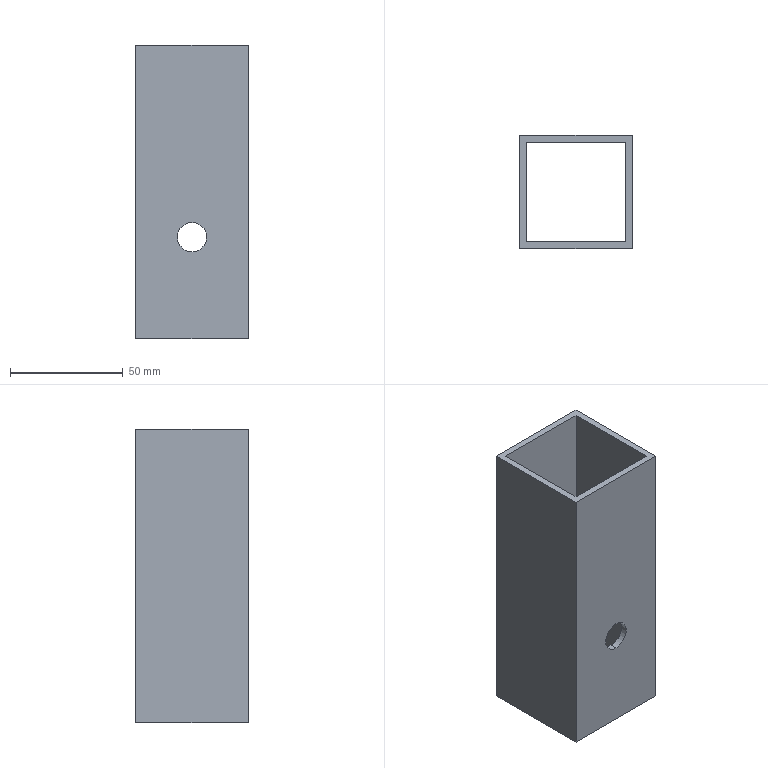Part | SolidWorks | features Cut 1, Extrusion 1 | 1 solid | 14 faces | box 50 x 50 x 130 mm | volume 72524 mm3 | plane 10 | cylinder 4 | commonest cylinder face diameters 13 x4
STEP:
#1=CARTESIAN_POINT('',(25.,0.,38.5));
#2=VERTEX_POINT('',#1);
#3=CARTESIAN_POINT('',(25.,0.,51.5));
#4=VERTEX_POINT('',#3);
#5=CARTESIAN_POINT('',(25.,0.,45.));
#6=DIRECTION('',(0.,1.,0.));
#7=DIRECTION('',(0.,0.,1.));
#8=AXIS2_PLACEMENT_3D('',#5,#6,#7);
#9=CIRCLE('',#8,6.5);
#10=EDGE_CURVE('',#2,#4,#9,.T.);
#11=ORIENTED_EDGE('',*,*,#10,.F.);
#12=CARTESIAN_POINT('',(25.,3.,38.5));
#13=VERTEX_POINT('',#12);
#14=CARTESIAN_POINT('',(25.,-80.,38.5));
#15=DIRECTION('',(0.,1.,0.));
#16=VECTOR('',#15,1000.);
#17=LINE('',#14,#16);
#18=EDGE_CURVE('',#2,#13,#17,.T.);
#19=ORIENTED_EDGE('',*,*,#18,.T.);
#20=CARTESIAN_POINT('',(25.,3.,51.5));
#21=VERTEX_POINT('',#20);
#22=CARTESIAN_POINT('',(25.,3.,45.));
#23=DIRECTION('',(0.,1.,0.));
#24=DIRECTION('',(0.,0.,1.));
#25=AXIS2_PLACEMENT_3D('',#22,#23,#24);
#26=CIRCLE('',#25,6.5);
#27=EDGE_CURVE('',#13,#21,#26,.T.);
#28=ORIENTED_EDGE('',*,*,#27,.T.);
#29=CARTESIAN_POINT('',(25.,-80.,51.5));
#30=DIRECTION('',(0.,1.,0.));
#31=VECTOR('',#30,1000.);
#32=LINE('',#29,#31);
#33=EDGE_CURVE('',#4,#21,#32,.T.);
#34=ORIENTED_EDGE('',*,*,#33,.F.);
#35=EDGE_LOOP('',(#11,#19,#28,#34));
#36=FACE_OUTER_BOUND('',#35,.T.);
#37=CARTESIAN_POINT('',(25.,-80.,45.));
#38=DIRECTION('',(0.,1.,0.));
#39=DIRECTION('',(0.,0.,1.));
#40=AXIS2_PLACEMENT_3D('',#37,#38,#39);
#41=CYLINDRICAL_SURFACE('',#40,6.5);
#42=ADVANCED_FACE('',(#36),#41,.F.);
#43=CARTESIAN_POINT('',(25.,47.,51.5));
#44=VERTEX_POINT('',#43);
#45=CARTESIAN_POINT('',(25.,47.,38.5));
#46=VERTEX_POINT('',#45);
#47=CARTESIAN_POINT('',(25.,47.,45.));
#48=DIRECTION('',(0.,-1.,0.));
#49=DIRECTION('',(0.,0.,-1.));
#50=AXIS2_PLACEMENT_3D('',#47,#48,#49);
#51=CIRCLE('',#50,6.5);
#52=EDGE_CURVE('',#44,#46,#51,.T.);
#53=ORIENTED_EDGE('',*,*,#52,.T.);
#54=CARTESIAN_POINT('',(25.,50.,38.5));
#55=VERTEX_POINT('',#54);
#56=CARTESIAN_POINT('',(25.,-80.,38.5));
#57=DIRECTION('',(0.,1.,0.));
#58=VECTOR('',#57,1000.);
#59=LINE('',#56,#58);
#60=EDGE_CURVE('',#46,#55,#59,.T.);
#61=ORIENTED_EDGE('',*,*,#60,.T.);
#62=CARTESIAN_POINT('',(25.,50.,51.5));
#63=VERTEX_POINT('',#62);
#64=CARTESIAN_POINT('',(25.,50.,45.));
#65=DIRECTION('',(0.,1.,0.));
#66=DIRECTION('',(0.,0.,1.));
#67=AXIS2_PLACEMENT_3D('',#64,#65,#66);
#68=CIRCLE('',#67,6.5);
#69=EDGE_CURVE('',#55,#63,#68,.T.);
#70=ORIENTED_EDGE('',*,*,#69,.T.);
#71=CARTESIAN_POINT('',(25.,-80.,51.5));
#72=DIRECTION('',(0.,1.,0.));
#73=VECTOR('',#72,1000.);
#74=LINE('',#71,#73);
#75=EDGE_CURVE('',#44,#63,#74,.T.);
#76=ORIENTED_EDGE('',*,*,#75,.F.);
#77=EDGE_LOOP('',(#53,#61,#70,#76));
#78=FACE_OUTER_BOUND('',#77,.T.);
#79=CARTESIAN_POINT('',(25.,-80.,45.));
#80=DIRECTION('',(0.,1.,0.));
#81=DIRECTION('',(0.,0.,1.));
#82=AXIS2_PLACEMENT_3D('',#79,#80,#81);
#83=CYLINDRICAL_SURFACE('',#82,6.5);
#84=ADVANCED_FACE('',(#78),#83,.F.);
#85=CARTESIAN_POINT('',(0.,0.,130.));
#86=VERTEX_POINT('',#85);
#87=CARTESIAN_POINT('',(50.,0.,130.));
#88=VERTEX_POINT('',#87);
#89=CARTESIAN_POINT('',(50.,0.,130.));
#90=DIRECTION('',(1.,0.,0.));
#91=VECTOR('',#90,1000.);
#92=LINE('',#89,#91);
#93=EDGE_CURVE('',#86,#88,#92,.T.);
#94=ORIENTED_EDGE('',*,*,#93,.T.);
#95=CARTESIAN_POINT('',(50.,50.,130.));
#96=VERTEX_POINT('',#95);
#97=CARTESIAN_POINT('',(50.,50.,130.));
#98=DIRECTION('',(0.,1.,0.));
#99=VECTOR('',#98,1000.);
#100=LINE('',#97,#99);
#101=EDGE_CURVE('',#88,#96,#100,.T.);
#102=ORIENTED_EDGE('',*,*,#101,.T.);
#103=CARTESIAN_POINT('',(0.,50.,130.));
#104=VERTEX_POINT('',#103);
#105=CARTESIAN_POINT('',(0.,50.,130.));
#106=DIRECTION('',(-1.,0.,0.));
#107=VECTOR('',#106,1000.);
#108=LINE('',#105,#107);
#109=EDGE_CURVE('',#96,#104,#108,.T.);
#110=ORIENTED_EDGE('',*,*,#109,.T.);
#111=CARTESIAN_POINT('',(0.,0.,130.));
#112=DIRECTION('',(0.,-1.,0.));
#113=VECTOR('',#112,1000.);
#114=LINE('',#111,#113);
#115=EDGE_CURVE('',#104,#86,#114,.T.);
#116=ORIENTED_EDGE('',*,*,#115,.T.);
#117=EDGE_LOOP('',(#94,#102,#110,#116));
#118=FACE_OUTER_BOUND('',#117,.T.);
#119=CARTESIAN_POINT('',(3.,3.,130.));
#120=VERTEX_POINT('',#119);
#121=CARTESIAN_POINT('',(47.,3.,130.));
#122=VERTEX_POINT('',#121);
#123=CARTESIAN_POINT('',(47.,3.,130.));
#124=DIRECTION('',(1.,0.,0.));
#125=VECTOR('',#124,1000.);
#126=LINE('',#123,#125);
#127=EDGE_CURVE('',#120,#122,#126,.T.);
#128=ORIENTED_EDGE('',*,*,#127,.F.);
#129=CARTESIAN_POINT('',(3.,47.,130.));
#130=VERTEX_POINT('',#129);
#131=CARTESIAN_POINT('',(3.,3.,130.));
#132=DIRECTION('',(0.,-1.,0.));
#133=VECTOR('',#132,1000.);
#134=LINE('',#131,#133);
#135=EDGE_CURVE('',#130,#120,#134,.T.);
#136=ORIENTED_EDGE('',*,*,#135,.F.);
#137=CARTESIAN_POINT('',(47.,47.,130.));
#138=VERTEX_POINT('',#137);
#139=CARTESIAN_POINT('',(3.,47.,130.));
#140=DIRECTION('',(-1.,0.,0.));
#141=VECTOR('',#140,1000.);
#142=LINE('',#139,#141);
#143=EDGE_CURVE('',#138,#130,#142,.T.);
#144=ORIENTED_EDGE('',*,*,#143,.F.);
#145=CARTESIAN_POINT('',(47.,47.,130.));
#146=DIRECTION('',(0.,1.,0.));
#147=VECTOR('',#146,1000.);
#148=LINE('',#145,#147);
#149=EDGE_CURVE('',#122,#138,#148,.T.);
#150=ORIENTED_EDGE('',*,*,#149,.F.);
#151=EDGE_LOOP('',(#128,#136,#144,#150));
#152=FACE_BOUND('',#151,.T.);
#153=CARTESIAN_POINT('',(0.,0.,130.));
#154=DIRECTION('',(0.,0.,-1.));
#155=DIRECTION('',(-1.,0.,0.));
#156=AXIS2_PLACEMENT_3D('',#153,#154,#155);
#157=PLANE('',#156);
#158=ADVANCED_FACE('',(#118,#152),#157,.F.);
#159=CARTESIAN_POINT('',(0.,0.,0.));
#160=VERTEX_POINT('',#159);
#161=CARTESIAN_POINT('',(50.,0.,0.));
#162=VERTEX_POINT('',#161);
#163=CARTESIAN_POINT('',(50.,0.,0.));
#164=DIRECTION('',(1.,0.,0.));
#165=VECTOR('',#164,1000.);
#166=LINE('',#163,#165);
#167=EDGE_CURVE('',#160,#162,#166,.T.);
#168=ORIENTED_EDGE('',*,*,#167,.F.);
#169=CARTESIAN_POINT('',(0.,50.,0.));
#170=VERTEX_POINT('',#169);
#171=CARTESIAN_POINT('',(0.,0.,0.));
#172=DIRECTION('',(0.,-1.,0.));
#173=VECTOR('',#172,1000.);
#174=LINE('',#171,#173);
#175=EDGE_CURVE('',#170,#160,#174,.T.);
#176=ORIENTED_EDGE('',*,*,#175,.F.);
#177=CARTESIAN_POINT('',(50.,50.,0.));
#178=VERTEX_POINT('',#177);
#179=CARTESIAN_POINT('',(0.,50.,0.));
#180=DIRECTION('',(-1.,0.,0.));
#181=VECTOR('',#180,1000.);
#182=LINE('',#179,#181);
#183=EDGE_CURVE('',#178,#170,#182,.T.);
#184=ORIENTED_EDGE('',*,*,#183,.F.);
#185=CARTESIAN_POINT('',(50.,50.,0.));
#186=DIRECTION('',(0.,1.,0.));
#187=VECTOR('',#186,1000.);
#188=LINE('',#185,#187);
#189=EDGE_CURVE('',#162,#178,#188,.T.);
#190=ORIENTED_EDGE('',*,*,#189,.F.);
#191=EDGE_LOOP('',(#168,#176,#184,#190));
#192=FACE_OUTER_BOUND('',#191,.T.);
#193=CARTESIAN_POINT('',(3.,47.,0.));
#194=VERTEX_POINT('',#193);
#195=CARTESIAN_POINT('',(3.,3.,0.));
#196=VERTEX_POINT('',#195);
#197=CARTESIAN_POINT('',(3.,3.,0.));
#198=DIRECTION('',(0.,-1.,0.));
#199=VECTOR('',#198,1000.);
#200=LINE('',#197,#199);
#201=EDGE_CURVE('',#194,#196,#200,.T.);
#202=ORIENTED_EDGE('',*,*,#201,.T.);
#203=CARTESIAN_POINT('',(47.,3.,0.));
#204=VERTEX_POINT('',#203);
#205=CARTESIAN_POINT('',(47.,3.,0.));
#206=DIRECTION('',(1.,0.,0.));
#207=VECTOR('',#206,1000.);
#208=LINE('',#205,#207);
#209=EDGE_CURVE('',#196,#204,#208,.T.);
#210=ORIENTED_EDGE('',*,*,#209,.T.);
#211=CARTESIAN_POINT('',(47.,47.,0.));
#212=VERTEX_POINT('',#211);
#213=CARTESIAN_POINT('',(47.,47.,0.));
#214=DIRECTION('',(0.,1.,0.));
#215=VECTOR('',#214,1000.);
#216=LINE('',#213,#215);
#217=EDGE_CURVE('',#204,#212,#216,.T.);
#218=ORIENTED_EDGE('',*,*,#217,.T.);
#219=CARTESIAN_POINT('',(3.,47.,0.));
#220=DIRECTION('',(-1.,0.,0.));
#221=VECTOR('',#220,1000.);
#222=LINE('',#219,#221);
#223=EDGE_CURVE('',#212,#194,#222,.T.);
#224=ORIENTED_EDGE('',*,*,#223,.T.);
#225=EDGE_LOOP('',(#202,#210,#218,#224));
#226=FACE_BOUND('',#225,.T.);
#227=CARTESIAN_POINT('',(0.,0.,0.));
#228=DIRECTION('',(0.,0.,-1.));
#229=DIRECTION('',(-1.,0.,0.));
#230=AXIS2_PLACEMENT_3D('',#227,#228,#229);
#231=PLANE('',#230);
#232=ADVANCED_FACE('',(#192,#226),#231,.T.);
#233=CARTESIAN_POINT('',(25.,0.,45.));
#234=DIRECTION('',(0.,1.,0.));
#235=DIRECTION('',(0.,0.,1.));
#236=AXIS2_PLACEMENT_3D('',#233,#234,#235);
#237=CIRCLE('',#236,6.5);
#238=EDGE_CURVE('',#4,#2,#237,.T.);
#239=ORIENTED_EDGE('',*,*,#238,.T.);
#240=ORIENTED_EDGE('',*,*,#10,.T.);
#241=EDGE_LOOP('',(#239,#240));
#242=FACE_BOUND('',#241,.T.);
#243=ORIENTED_EDGE('',*,*,#167,.T.);
#244=CARTESIAN_POINT('',(50.,0.,130.));
#245=DIRECTION('',(0.,0.,-1.));
#246=VECTOR('',#245,1000.);
#247=LINE('',#244,#246);
#248=EDGE_CURVE('',#88,#162,#247,.T.);
#249=ORIENTED_EDGE('',*,*,#248,.F.);
#250=ORIENTED_EDGE('',*,*,#93,.F.);
#251=CARTESIAN_POINT('',(0.,0.,130.));
#252=DIRECTION('',(0.,0.,-1.));
#253=VECTOR('',#252,1000.);
#254=LINE('',#251,#253);
#255=EDGE_CURVE('',#86,#160,#254,.T.);
#256=ORIENTED_EDGE('',*,*,#255,.T.);
#257=EDGE_LOOP('',(#243,#249,#250,#256));
#258=FACE_OUTER_BOUND('',#257,.T.);
#259=CARTESIAN_POINT('',(50.,0.,130.));
#260=DIRECTION('',(0.,1.,0.));
#261=DIRECTION('',(0.,0.,1.));
#262=AXIS2_PLACEMENT_3D('',#259,#260,#261);
#263=PLANE('',#262);
#264=ADVANCED_FACE('',(#242,#258),#263,.F.);
#265=ORIENTED_EDGE('',*,*,#189,.T.);
#266=CARTESIAN_POINT('',(50.,50.,130.));
#267=DIRECTION('',(0.,0.,-1.));
#268=VECTOR('',#267,1000.);
#269=LINE('',#266,#268);
#270=EDGE_CURVE('',#96,#178,#269,.T.);
#271=ORIENTED_EDGE('',*,*,#270,.F.);
#272=ORIENTED_EDGE('',*,*,#101,.F.);
#273=ORIENTED_EDGE('',*,*,#248,.T.);
#274=EDGE_LOOP('',(#265,#271,#272,#273));
#275=FACE_OUTER_BOUND('',#274,.T.);
#276=CARTESIAN_POINT('',(50.,50.,130.));
#277=DIRECTION('',(-1.,0.,0.));
#278=DIRECTION('',(0.,0.,1.));
#279=AXIS2_PLACEMENT_3D('',#276,#277,#278);
#280=PLANE('',#279);
#281=ADVANCED_FACE('',(#275),#280,.F.);
#282=CARTESIAN_POINT('',(25.,50.,45.));
#283=DIRECTION('',(0.,1.,0.));
#284=DIRECTION('',(0.,0.,1.));
#285=AXIS2_PLACEMENT_3D('',#282,#283,#284);
#286=CIRCLE('',#285,6.5);
#287=EDGE_CURVE('',#63,#55,#286,.T.);
#288=ORIENTED_EDGE('',*,*,#287,.F.);
#289=ORIENTED_EDGE('',*,*,#69,.F.);
#290=EDGE_LOOP('',(#288,#289));
#291=FACE_BOUND('',#290,.T.);
#292=ORIENTED_EDGE('',*,*,#183,.T.);
#293=CARTESIAN_POINT('',(0.,50.,130.));
#294=DIRECTION('',(0.,0.,-1.));
#295=VECTOR('',#294,1000.);
#296=LINE('',#293,#295);
#297=EDGE_CURVE('',#104,#170,#296,.T.);
#298=ORIENTED_EDGE('',*,*,#297,.F.);
#299=ORIENTED_EDGE('',*,*,#109,.F.);
#300=ORIENTED_EDGE('',*,*,#270,.T.);
#301=EDGE_LOOP('',(#292,#298,#299,#300));
#302=FACE_OUTER_BOUND('',#301,.T.);
#303=CARTESIAN_POINT('',(0.,50.,130.));
#304=DIRECTION('',(0.,-1.,0.));
#305=DIRECTION('',(0.,0.,-1.));
#306=AXIS2_PLACEMENT_3D('',#303,#304,#305);
#307=PLANE('',#306);
#308=ADVANCED_FACE('',(#291,#302),#307,.F.);
#309=ORIENTED_EDGE('',*,*,#175,.T.);
#310=ORIENTED_EDGE('',*,*,#255,.F.);
#311=ORIENTED_EDGE('',*,*,#115,.F.);
#312=ORIENTED_EDGE('',*,*,#297,.T.);
#313=EDGE_LOOP('',(#309,#310,#311,#312));
#314=FACE_OUTER_BOUND('',#313,.T.);
#315=CARTESIAN_POINT('',(0.,0.,130.));
#316=DIRECTION('',(1.,0.,0.));
#317=DIRECTION('',(0.,0.,-1.));
#318=AXIS2_PLACEMENT_3D('',#315,#316,#317);
#319=PLANE('',#318);
#320=ADVANCED_FACE('',(#314),#319,.F.);
#321=CARTESIAN_POINT('',(25.,3.,45.));
#322=DIRECTION('',(0.,1.,0.));
#323=DIRECTION('',(0.,0.,1.));
#324=AXIS2_PLACEMENT_3D('',#321,#322,#323);
#325=CIRCLE('',#324,6.5);
#326=EDGE_CURVE('',#21,#13,#325,.T.);
#327=ORIENTED_EDGE('',*,*,#326,.F.);
#328=ORIENTED_EDGE('',*,*,#27,.F.);
#329=EDGE_LOOP('',(#327,#328));
#330=FACE_BOUND('',#329,.T.);
#331=ORIENTED_EDGE('',*,*,#209,.F.);
#332=CARTESIAN_POINT('',(3.,3.,130.));
#333=DIRECTION('',(0.,0.,-1.));
#334=VECTOR('',#333,1000.);
#335=LINE('',#332,#334);
#336=EDGE_CURVE('',#120,#196,#335,.T.);
#337=ORIENTED_EDGE('',*,*,#336,.F.);
#338=ORIENTED_EDGE('',*,*,#127,.T.);
#339=CARTESIAN_POINT('',(47.,3.,130.));
#340=DIRECTION('',(0.,0.,-1.));
#341=VECTOR('',#340,1000.);
#342=LINE('',#339,#341);
#343=EDGE_CURVE('',#122,#204,#342,.T.);
#344=ORIENTED_EDGE('',*,*,#343,.T.);
#345=EDGE_LOOP('',(#331,#337,#338,#344));
#346=FACE_OUTER_BOUND('',#345,.T.);
#347=CARTESIAN_POINT('',(47.,3.,130.));
#348=DIRECTION('',(0.,1.,0.));
#349=DIRECTION('',(0.,0.,1.));
#350=AXIS2_PLACEMENT_3D('',#347,#348,#349);
#351=PLANE('',#350);
#352=ADVANCED_FACE('',(#330,#346),#351,.T.);
#353=ORIENTED_EDGE('',*,*,#217,.F.);
#354=ORIENTED_EDGE('',*,*,#343,.F.);
#355=ORIENTED_EDGE('',*,*,#149,.T.);
#356=CARTESIAN_POINT('',(47.,47.,130.));
#357=DIRECTION('',(0.,0.,-1.));
#358=VECTOR('',#357,1000.);
#359=LINE('',#356,#358);
#360=EDGE_CURVE('',#138,#212,#359,.T.);
#361=ORIENTED_EDGE('',*,*,#360,.T.);
#362=EDGE_LOOP('',(#353,#354,#355,#361));
#363=FACE_OUTER_BOUND('',#362,.T.);
#364=CARTESIAN_POINT('',(47.,47.,130.));
#365=DIRECTION('',(-1.,0.,0.));
#366=DIRECTION('',(0.,0.,1.));
#367=AXIS2_PLACEMENT_3D('',#364,#365,#366);
#368=PLANE('',#367);
#369=ADVANCED_FACE('',(#363),#368,.T.);
#370=ORIENTED_EDGE('',*,*,#52,.F.);
#371=CARTESIAN_POINT('',(25.,47.,45.));
#372=DIRECTION('',(0.,-1.,0.));
#373=DIRECTION('',(0.,0.,-1.));
#374=AXIS2_PLACEMENT_3D('',#371,#372,#373);
#375=CIRCLE('',#374,6.5);
#376=EDGE_CURVE('',#46,#44,#375,.T.);
#377=ORIENTED_EDGE('',*,*,#376,.F.);
#378=EDGE_LOOP('',(#370,#377));
#379=FACE_BOUND('',#378,.T.);
#380=ORIENTED_EDGE('',*,*,#223,.F.);
#381=ORIENTED_EDGE('',*,*,#360,.F.);
#382=ORIENTED_EDGE('',*,*,#143,.T.);
#383=CARTESIAN_POINT('',(3.,47.,130.));
#384=DIRECTION('',(0.,0.,-1.));
#385=VECTOR('',#384,1000.);
#386=LINE('',#383,#385);
#387=EDGE_CURVE('',#130,#194,#386,.T.);
#388=ORIENTED_EDGE('',*,*,#387,.T.);
#389=EDGE_LOOP('',(#380,#381,#382,#388));
#390=FACE_OUTER_BOUND('',#389,.T.);
#391=CARTESIAN_POINT('',(3.,47.,130.));
#392=DIRECTION('',(0.,-1.,0.));
#393=DIRECTION('',(0.,0.,-1.));
#394=AXIS2_PLACEMENT_3D('',#391,#392,#393);
#395=PLANE('',#394);
#396=ADVANCED_FACE('',(#379,#390),#395,.T.);
#397=ORIENTED_EDGE('',*,*,#201,.F.);
#398=ORIENTED_EDGE('',*,*,#387,.F.);
#399=ORIENTED_EDGE('',*,*,#135,.T.);
#400=ORIENTED_EDGE('',*,*,#336,.T.);
#401=EDGE_LOOP('',(#397,#398,#399,#400));
#402=FACE_OUTER_BOUND('',#401,.T.);
#403=CARTESIAN_POINT('',(3.,3.,130.));
#404=DIRECTION('',(1.,0.,0.));
#405=DIRECTION('',(0.,0.,-1.));
#406=AXIS2_PLACEMENT_3D('',#403,#404,#405);
#407=PLANE('',#406);
#408=ADVANCED_FACE('',(#402),#407,.T.);
#409=ORIENTED_EDGE('',*,*,#60,.F.);
#410=ORIENTED_EDGE('',*,*,#376,.T.);
#411=ORIENTED_EDGE('',*,*,#75,.T.);
#412=ORIENTED_EDGE('',*,*,#287,.T.);
#413=EDGE_LOOP('',(#409,#410,#411,#412));
#414=FACE_OUTER_BOUND('',#413,.T.);
#415=CARTESIAN_POINT('',(25.,-80.,45.));
#416=DIRECTION('',(0.,1.,0.));
#417=DIRECTION('',(0.,0.,1.));
#418=AXIS2_PLACEMENT_3D('',#415,#416,#417);
#419=CYLINDRICAL_SURFACE('',#418,6.5);
#420=ADVANCED_FACE('',(#414),#419,.F.);
#421=ORIENTED_EDGE('',*,*,#18,.F.);
#422=ORIENTED_EDGE('',*,*,#238,.F.);
#423=ORIENTED_EDGE('',*,*,#33,.T.);
#424=ORIENTED_EDGE('',*,*,#326,.T.);
#425=EDGE_LOOP('',(#421,#422,#423,#424));
#426=FACE_OUTER_BOUND('',#425,.T.);
#427=CARTESIAN_POINT('',(25.,-80.,45.));
#428=DIRECTION('',(0.,1.,0.));
#429=DIRECTION('',(0.,0.,1.));
#430=AXIS2_PLACEMENT_3D('',#427,#428,#429);
#431=CYLINDRICAL_SURFACE('',#430,6.5);
#432=ADVANCED_FACE('',(#426),#431,.F.);
#433=CLOSED_SHELL('',(#42,#84,#158,#232,#264,#281,#308,#320,#352,#369,#396,#408,#420,#432));
#434=MANIFOLD_SOLID_BREP('',#433);
#435=CARTESIAN_POINT('',(0.,0.,0.));
#436=DIRECTION('',(0.,0.,1.));
#437=DIRECTION('',(1.,0.,0.));
#438=AXIS2_PLACEMENT_3D('',#435,#436,#437);
#439=(LENGTH_UNIT()NAMED_UNIT(*)SI_UNIT(.MILLI.,.METRE.));
#440=UNCERTAINTY_MEASURE_WITH_UNIT(LENGTH_MEASURE(0.00001),#439,'','');
#441=(NAMED_UNIT(*)PLANE_ANGLE_UNIT()SI_UNIT($,.RADIAN.));
#442=(NAMED_UNIT(*)SI_UNIT($,.STERADIAN.)SOLID_ANGLE_UNIT());
#443=(GEOMETRIC_REPRESENTATION_CONTEXT(3)GLOBAL_UNCERTAINTY_ASSIGNED_CONTEXT((#440))GLOBAL_UNIT_ASSIGNED_CONTEXT((#439,#441,#442))REPRESENTATION_CONTEXT('',''));
#444=ADVANCED_BREP_SHAPE_REPRESENTATION('',(#434,#438),#443);